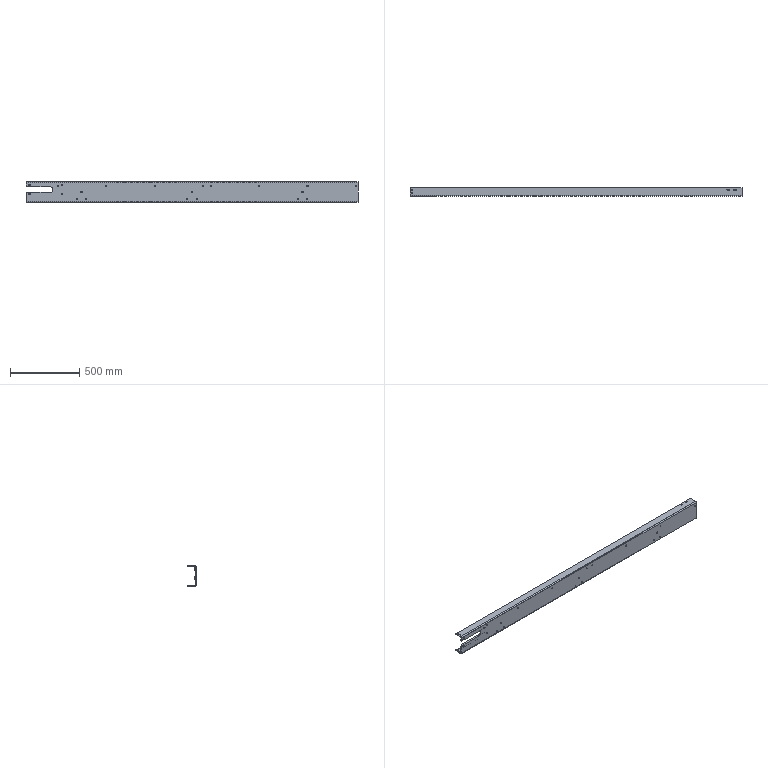Part | STEP file | UPPER.FRAME.IDEL.SIDE.2.stp | 1 solid | 111 faces | box 2400 x 60 x 150 mm | volume 2840221 mm3 | cylinder 52 | spline 48 | plane 11 | commonest cylinder face diameters 8 x20 10 x12 7 x10 9 x8 40 x2